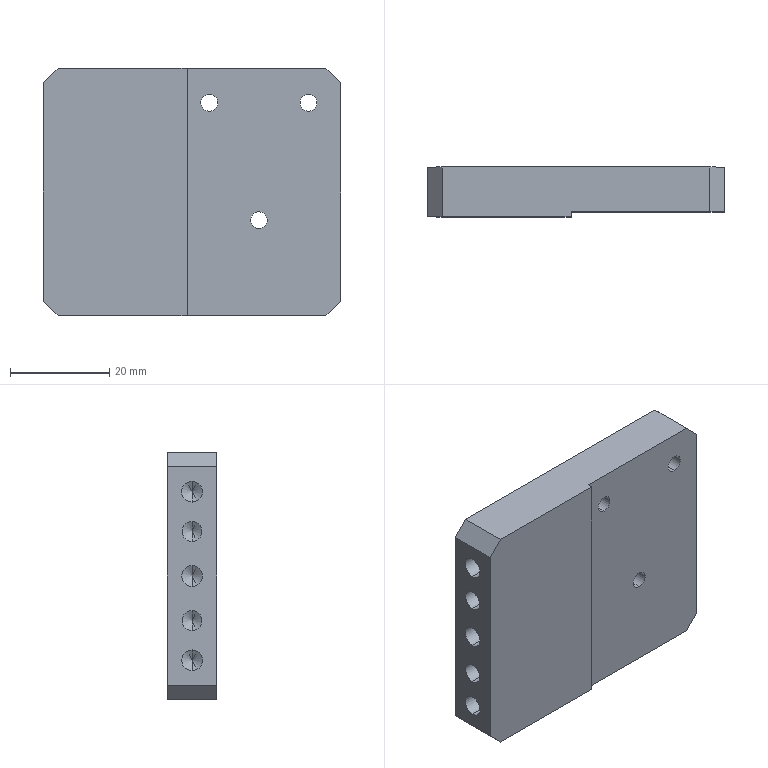Part | SolidWorks | features HoleWzd 3, Chamfer 1, Extrusion 1, ICE 1 | 1 solid | 47 faces | box 60 x 10 x 50 mm | volume 26983 mm3 | cylinder 22 | plane 15 | cone 10 | commonest cylinder face diameters 3.4 x6 4.2 x6 6 x6 4 x4
STEP:
#1=CARTESIAN_POINT('',(-17.6,5.,7.));
#2=VERTEX_POINT('',#1);
#3=CARTESIAN_POINT('',(-17.6,5.,11.));
#4=VERTEX_POINT('',#3);
#5=CARTESIAN_POINT('',(-17.6,5.,9.));
#6=DIRECTION('',(-1.,0.,0.));
#7=DIRECTION('',(0.,0.,1.));
#8=AXIS2_PLACEMENT_3D('',#5,#6,#7);
#9=CIRCLE('',#8,2.);
#10=EDGE_CURVE('',#2,#4,#9,.T.);
#11=ORIENTED_EDGE('',*,*,#10,.F.);
#12=CARTESIAN_POINT('',(-30.,5.,7.));
#13=VERTEX_POINT('',#12);
#14=CARTESIAN_POINT('',(-30.,5.,7.));
#15=DIRECTION('',(-1.,0.,0.));
#16=VECTOR('',#15,1000.);
#17=LINE('',#14,#16);
#18=EDGE_CURVE('',#2,#13,#17,.T.);
#19=ORIENTED_EDGE('',*,*,#18,.T.);
#20=CARTESIAN_POINT('',(-30.,5.,11.));
#21=VERTEX_POINT('',#20);
#22=CARTESIAN_POINT('',(-30.,5.,9.));
#23=DIRECTION('',(-1.,0.,0.));
#24=DIRECTION('',(0.,0.,1.));
#25=AXIS2_PLACEMENT_3D('',#22,#23,#24);
#26=CIRCLE('',#25,2.);
#27=EDGE_CURVE('',#13,#21,#26,.T.);
#28=ORIENTED_EDGE('',*,*,#27,.T.);
#29=CARTESIAN_POINT('',(-30.,5.,11.));
#30=DIRECTION('',(-1.,0.,0.));
#31=VECTOR('',#30,1000.);
#32=LINE('',#29,#31);
#33=EDGE_CURVE('',#4,#21,#32,.T.);
#34=ORIENTED_EDGE('',*,*,#33,.F.);
#35=EDGE_LOOP('',(#11,#19,#28,#34));
#36=FACE_OUTER_BOUND('',#35,.T.);
#37=CARTESIAN_POINT('',(-30.,5.,9.));
#38=DIRECTION('',(-1.,0.,0.));
#39=DIRECTION('',(0.,0.,1.));
#40=AXIS2_PLACEMENT_3D('',#37,#38,#39);
#41=CYLINDRICAL_SURFACE('',#40,2.);
#42=ADVANCED_FACE('',(#36),#41,.F.);
#43=CARTESIAN_POINT('',(-16.398,5.,9.));
#44=VERTEX_POINT('',#43);
#45=CARTESIAN_POINT('',(-17.6,5.,11.));
#46=DIRECTION('',(-0.515,0.,0.8572));
#47=VECTOR('',#46,1000.);
#48=LINE('',#45,#47);
#49=EDGE_CURVE('',#44,#4,#48,.T.);
#50=ORIENTED_EDGE('',*,*,#49,.F.);
#51=CARTESIAN_POINT('',(-17.6,5.,7.));
#52=DIRECTION('',(-0.515,0.,-0.8572));
#53=VECTOR('',#52,1000.);
#54=LINE('',#51,#53);
#55=EDGE_CURVE('',#44,#2,#54,.T.);
#56=ORIENTED_EDGE('',*,*,#55,.T.);
#57=ORIENTED_EDGE('',*,*,#10,.T.);
#58=EDGE_LOOP('',(#50,#56,#57));
#59=FACE_OUTER_BOUND('',#58,.T.);
#60=CARTESIAN_POINT('',(-17.6,5.,9.));
#61=DIRECTION('',(-1.,0.,0.));
#62=DIRECTION('',(0.,0.,1.));
#63=AXIS2_PLACEMENT_3D('',#60,#61,#62);
#64=CONICAL_SURFACE('',#63,2.,1.03);
#65=ADVANCED_FACE('',(#59),#64,.F.);
#66=CARTESIAN_POINT('',(-17.6,5.,-11.));
#67=VERTEX_POINT('',#66);
#68=CARTESIAN_POINT('',(-17.6,5.,-7.));
#69=VERTEX_POINT('',#68);
#70=CARTESIAN_POINT('',(-17.6,5.,-9.));
#71=DIRECTION('',(-1.,0.,0.));
#72=DIRECTION('',(0.,0.,1.));
#73=AXIS2_PLACEMENT_3D('',#70,#71,#72);
#74=CIRCLE('',#73,2.);
#75=EDGE_CURVE('',#67,#69,#74,.T.);
#76=ORIENTED_EDGE('',*,*,#75,.F.);
#77=CARTESIAN_POINT('',(-30.,5.,-11.));
#78=VERTEX_POINT('',#77);
#79=CARTESIAN_POINT('',(-30.,5.,-11.));
#80=DIRECTION('',(-1.,0.,0.));
#81=VECTOR('',#80,1000.);
#82=LINE('',#79,#81);
#83=EDGE_CURVE('',#67,#78,#82,.T.);
#84=ORIENTED_EDGE('',*,*,#83,.T.);
#85=CARTESIAN_POINT('',(-30.,5.,-7.));
#86=VERTEX_POINT('',#85);
#87=CARTESIAN_POINT('',(-30.,5.,-9.));
#88=DIRECTION('',(-1.,0.,0.));
#89=DIRECTION('',(0.,0.,1.));
#90=AXIS2_PLACEMENT_3D('',#87,#88,#89);
#91=CIRCLE('',#90,2.);
#92=EDGE_CURVE('',#78,#86,#91,.T.);
#93=ORIENTED_EDGE('',*,*,#92,.T.);
#94=CARTESIAN_POINT('',(-30.,5.,-7.));
#95=DIRECTION('',(-1.,0.,0.));
#96=VECTOR('',#95,1000.);
#97=LINE('',#94,#96);
#98=EDGE_CURVE('',#69,#86,#97,.T.);
#99=ORIENTED_EDGE('',*,*,#98,.F.);
#100=EDGE_LOOP('',(#76,#84,#93,#99));
#101=FACE_OUTER_BOUND('',#100,.T.);
#102=CARTESIAN_POINT('',(-30.,5.,-9.));
#103=DIRECTION('',(-1.,0.,0.));
#104=DIRECTION('',(0.,0.,1.));
#105=AXIS2_PLACEMENT_3D('',#102,#103,#104);
#106=CYLINDRICAL_SURFACE('',#105,2.);
#107=ADVANCED_FACE('',(#101),#106,.F.);
#108=CARTESIAN_POINT('',(-16.398,5.,-9.));
#109=VERTEX_POINT('',#108);
#110=CARTESIAN_POINT('',(-17.6,5.,-7.));
#111=DIRECTION('',(-0.515,0.,0.8572));
#112=VECTOR('',#111,1000.);
#113=LINE('',#110,#112);
#114=EDGE_CURVE('',#109,#69,#113,.T.);
#115=ORIENTED_EDGE('',*,*,#114,.F.);
#116=CARTESIAN_POINT('',(-17.6,5.,-11.));
#117=DIRECTION('',(-0.515,0.,-0.8572));
#118=VECTOR('',#117,1000.);
#119=LINE('',#116,#118);
#120=EDGE_CURVE('',#109,#67,#119,.T.);
#121=ORIENTED_EDGE('',*,*,#120,.T.);
#122=ORIENTED_EDGE('',*,*,#75,.T.);
#123=EDGE_LOOP('',(#115,#121,#122));
#124=FACE_OUTER_BOUND('',#123,.T.);
#125=CARTESIAN_POINT('',(-17.6,5.,-9.));
#126=DIRECTION('',(-1.,0.,0.));
#127=DIRECTION('',(0.,0.,1.));
#128=AXIS2_PLACEMENT_3D('',#125,#126,#127);
#129=CONICAL_SURFACE('',#128,2.,1.03);
#130=ADVANCED_FACE('',(#124),#129,.F.);
#131=CARTESIAN_POINT('',(23.5,6.6,15.));
#132=VERTEX_POINT('',#131);
#133=CARTESIAN_POINT('',(23.5,6.6,21.));
#134=VERTEX_POINT('',#133);
#135=CARTESIAN_POINT('',(23.5,6.6,18.));
#136=DIRECTION('',(0.,1.,0.));
#137=DIRECTION('',(0.,0.,1.));
#138=AXIS2_PLACEMENT_3D('',#135,#136,#137);
#139=CIRCLE('',#138,3.);
#140=EDGE_CURVE('',#132,#134,#139,.T.);
#141=ORIENTED_EDGE('',*,*,#140,.F.);
#142=CARTESIAN_POINT('',(23.5,10.,15.));
#143=VERTEX_POINT('',#142);
#144=CARTESIAN_POINT('',(23.5,10.,15.));
#145=DIRECTION('',(0.,1.,0.));
#146=VECTOR('',#145,1000.);
#147=LINE('',#144,#146);
#148=EDGE_CURVE('',#132,#143,#147,.T.);
#149=ORIENTED_EDGE('',*,*,#148,.T.);
#150=CARTESIAN_POINT('',(23.5,10.,21.));
#151=VERTEX_POINT('',#150);
#152=CARTESIAN_POINT('',(23.5,10.,18.));
#153=DIRECTION('',(0.,1.,0.));
#154=DIRECTION('',(0.,0.,1.));
#155=AXIS2_PLACEMENT_3D('',#152,#153,#154);
#156=CIRCLE('',#155,3.);
#157=EDGE_CURVE('',#143,#151,#156,.T.);
#158=ORIENTED_EDGE('',*,*,#157,.T.);
#159=CARTESIAN_POINT('',(23.5,10.,21.));
#160=DIRECTION('',(0.,1.,0.));
#161=VECTOR('',#160,1000.);
#162=LINE('',#159,#161);
#163=EDGE_CURVE('',#134,#151,#162,.T.);
#164=ORIENTED_EDGE('',*,*,#163,.F.);
#165=EDGE_LOOP('',(#141,#149,#158,#164));
#166=FACE_OUTER_BOUND('',#165,.T.);
#167=CARTESIAN_POINT('',(23.5,10.,18.));
#168=DIRECTION('',(0.,1.,0.));
#169=DIRECTION('',(0.,0.,1.));
#170=AXIS2_PLACEMENT_3D('',#167,#168,#169);
#171=CYLINDRICAL_SURFACE('',#170,3.);
#172=ADVANCED_FACE('',(#166),#171,.F.);
#173=CARTESIAN_POINT('',(23.5,1.,19.7));
#174=VERTEX_POINT('',#173);
#175=CARTESIAN_POINT('',(23.5,1.,16.3));
#176=VERTEX_POINT('',#175);
#177=CARTESIAN_POINT('',(23.5,1.,18.));
#178=DIRECTION('',(0.,-1.,0.));
#179=DIRECTION('',(0.,0.,-1.));
#180=AXIS2_PLACEMENT_3D('',#177,#178,#179);
#181=CIRCLE('',#180,1.7);
#182=EDGE_CURVE('',#174,#176,#181,.T.);
#183=ORIENTED_EDGE('',*,*,#182,.T.);
#184=CARTESIAN_POINT('',(23.5,6.6,16.3));
#185=VERTEX_POINT('',#184);
#186=CARTESIAN_POINT('',(23.5,10.,16.3));
#187=DIRECTION('',(0.,1.,0.));
#188=VECTOR('',#187,1000.);
#189=LINE('',#186,#188);
#190=EDGE_CURVE('',#176,#185,#189,.T.);
#191=ORIENTED_EDGE('',*,*,#190,.T.);
#192=CARTESIAN_POINT('',(23.5,6.6,19.7));
#193=VERTEX_POINT('',#192);
#194=CARTESIAN_POINT('',(23.5,6.6,18.));
#195=DIRECTION('',(0.,1.,0.));
#196=DIRECTION('',(0.,0.,1.));
#197=AXIS2_PLACEMENT_3D('',#194,#195,#196);
#198=CIRCLE('',#197,1.7);
#199=EDGE_CURVE('',#185,#193,#198,.T.);
#200=ORIENTED_EDGE('',*,*,#199,.T.);
#201=CARTESIAN_POINT('',(23.5,10.,19.7));
#202=DIRECTION('',(0.,1.,0.));
#203=VECTOR('',#202,1000.);
#204=LINE('',#201,#203);
#205=EDGE_CURVE('',#174,#193,#204,.T.);
#206=ORIENTED_EDGE('',*,*,#205,.F.);
#207=EDGE_LOOP('',(#183,#191,#200,#206));
#208=FACE_OUTER_BOUND('',#207,.T.);
#209=CARTESIAN_POINT('',(23.5,10.,18.));
#210=DIRECTION('',(0.,1.,0.));
#211=DIRECTION('',(0.,0.,1.));
#212=AXIS2_PLACEMENT_3D('',#209,#210,#211);
#213=CYLINDRICAL_SURFACE('',#212,1.7);
#214=ADVANCED_FACE('',(#208),#213,.F.);
#215=CARTESIAN_POINT('',(3.5,6.6,15.));
#216=VERTEX_POINT('',#215);
#217=CARTESIAN_POINT('',(3.5,6.6,21.));
#218=VERTEX_POINT('',#217);
#219=CARTESIAN_POINT('',(3.5,6.6,18.));
#220=DIRECTION('',(0.,1.,0.));
#221=DIRECTION('',(0.,0.,1.));
#222=AXIS2_PLACEMENT_3D('',#219,#220,#221);
#223=CIRCLE('',#222,3.);
#224=EDGE_CURVE('',#216,#218,#223,.T.);
#225=ORIENTED_EDGE('',*,*,#224,.F.);
#226=CARTESIAN_POINT('',(3.5,10.,15.));
#227=VERTEX_POINT('',#226);
#228=CARTESIAN_POINT('',(3.5,10.,15.));
#229=DIRECTION('',(0.,1.,0.));
#230=VECTOR('',#229,1000.);
#231=LINE('',#228,#230);
#232=EDGE_CURVE('',#216,#227,#231,.T.);
#233=ORIENTED_EDGE('',*,*,#232,.T.);
#234=CARTESIAN_POINT('',(3.5,10.,21.));
#235=VERTEX_POINT('',#234);
#236=CARTESIAN_POINT('',(3.5,10.,18.));
#237=DIRECTION('',(0.,1.,0.));
#238=DIRECTION('',(0.,0.,1.));
#239=AXIS2_PLACEMENT_3D('',#236,#237,#238);
#240=CIRCLE('',#239,3.);
#241=EDGE_CURVE('',#227,#235,#240,.T.);
#242=ORIENTED_EDGE('',*,*,#241,.T.);
#243=CARTESIAN_POINT('',(3.5,10.,21.));
#244=DIRECTION('',(0.,1.,0.));
#245=VECTOR('',#244,1000.);
#246=LINE('',#243,#245);
#247=EDGE_CURVE('',#218,#235,#246,.T.);
#248=ORIENTED_EDGE('',*,*,#247,.F.);
#249=EDGE_LOOP('',(#225,#233,#242,#248));
#250=FACE_OUTER_BOUND('',#249,.T.);
#251=CARTESIAN_POINT('',(3.5,10.,18.));
#252=DIRECTION('',(0.,1.,0.));
#253=DIRECTION('',(0.,0.,1.));
#254=AXIS2_PLACEMENT_3D('',#251,#252,#253);
#255=CYLINDRICAL_SURFACE('',#254,3.);
#256=ADVANCED_FACE('',(#250),#255,.F.);
#257=CARTESIAN_POINT('',(3.5,1.,19.7));
#258=VERTEX_POINT('',#257);
#259=CARTESIAN_POINT('',(3.5,1.,16.3));
#260=VERTEX_POINT('',#259);
#261=CARTESIAN_POINT('',(3.5,1.,18.));
#262=DIRECTION('',(0.,-1.,0.));
#263=DIRECTION('',(0.,0.,-1.));
#264=AXIS2_PLACEMENT_3D('',#261,#262,#263);
#265=CIRCLE('',#264,1.7);
#266=EDGE_CURVE('',#258,#260,#265,.T.);
#267=ORIENTED_EDGE('',*,*,#266,.T.);
#268=CARTESIAN_POINT('',(3.5,6.6,16.3));
#269=VERTEX_POINT('',#268);
#270=CARTESIAN_POINT('',(3.5,10.,16.3));
#271=DIRECTION('',(0.,1.,0.));
#272=VECTOR('',#271,1000.);
#273=LINE('',#270,#272);
#274=EDGE_CURVE('',#260,#269,#273,.T.);
#275=ORIENTED_EDGE('',*,*,#274,.T.);
#276=CARTESIAN_POINT('',(3.5,6.6,19.7));
#277=VERTEX_POINT('',#276);
#278=CARTESIAN_POINT('',(3.5,6.6,18.));
#279=DIRECTION('',(0.,1.,0.));
#280=DIRECTION('',(0.,0.,1.));
#281=AXIS2_PLACEMENT_3D('',#278,#279,#280);
#282=CIRCLE('',#281,1.7);
#283=EDGE_CURVE('',#269,#277,#282,.T.);
#284=ORIENTED_EDGE('',*,*,#283,.T.);
#285=CARTESIAN_POINT('',(3.5,10.,19.7));
#286=DIRECTION('',(0.,1.,0.));
#287=VECTOR('',#286,1000.);
#288=LINE('',#285,#287);
#289=EDGE_CURVE('',#258,#277,#288,.T.);
#290=ORIENTED_EDGE('',*,*,#289,.F.);
#291=EDGE_LOOP('',(#267,#275,#284,#290));
#292=FACE_OUTER_BOUND('',#291,.T.);
#293=CARTESIAN_POINT('',(3.5,10.,18.));
#294=DIRECTION('',(0.,1.,0.));
#295=DIRECTION('',(0.,0.,1.));
#296=AXIS2_PLACEMENT_3D('',#293,#294,#295);
#297=CYLINDRICAL_SURFACE('',#296,1.7);
#298=ADVANCED_FACE('',(#292),#297,.F.);
#299=CARTESIAN_POINT('',(13.5,6.6,-8.7));
#300=VERTEX_POINT('',#299);
#301=CARTESIAN_POINT('',(13.5,6.6,-2.7));
#302=VERTEX_POINT('',#301);
#303=CARTESIAN_POINT('',(13.5,6.6,-5.7));
#304=DIRECTION('',(0.,1.,0.));
#305=DIRECTION('',(0.,0.,1.));
#306=AXIS2_PLACEMENT_3D('',#303,#304,#305);
#307=CIRCLE('',#306,3.);
#308=EDGE_CURVE('',#300,#302,#307,.T.);
#309=ORIENTED_EDGE('',*,*,#308,.F.);
#310=CARTESIAN_POINT('',(13.5,10.,-8.7));
#311=VERTEX_POINT('',#310);
#312=CARTESIAN_POINT('',(13.5,10.,-8.7));
#313=DIRECTION('',(0.,1.,0.));
#314=VECTOR('',#313,1000.);
#315=LINE('',#312,#314);
#316=EDGE_CURVE('',#300,#311,#315,.T.);
#317=ORIENTED_EDGE('',*,*,#316,.T.);
#318=CARTESIAN_POINT('',(13.5,10.,-2.7));
#319=VERTEX_POINT('',#318);
#320=CARTESIAN_POINT('',(13.5,10.,-5.7));
#321=DIRECTION('',(0.,1.,0.));
#322=DIRECTION('',(0.,0.,1.));
#323=AXIS2_PLACEMENT_3D('',#320,#321,#322);
#324=CIRCLE('',#323,3.);
#325=EDGE_CURVE('',#311,#319,#324,.T.);
#326=ORIENTED_EDGE('',*,*,#325,.T.);
#327=CARTESIAN_POINT('',(13.5,10.,-2.7));
#328=DIRECTION('',(0.,1.,0.));
#329=VECTOR('',#328,1000.);
#330=LINE('',#327,#329);
#331=EDGE_CURVE('',#302,#319,#330,.T.);
#332=ORIENTED_EDGE('',*,*,#331,.F.);
#333=EDGE_LOOP('',(#309,#317,#326,#332));
#334=FACE_OUTER_BOUND('',#333,.T.);
#335=CARTESIAN_POINT('',(13.5,10.,-5.7));
#336=DIRECTION('',(0.,1.,0.));
#337=DIRECTION('',(0.,0.,1.));
#338=AXIS2_PLACEMENT_3D('',#335,#336,#337);
#339=CYLINDRICAL_SURFACE('',#338,3.);
#340=ADVANCED_FACE('',(#334),#339,.F.);
#341=CARTESIAN_POINT('',(13.5,1.,-4.));
#342=VERTEX_POINT('',#341);
#343=CARTESIAN_POINT('',(13.5,1.,-7.4));
#344=VERTEX_POINT('',#343);
#345=CARTESIAN_POINT('',(13.5,1.,-5.7));
#346=DIRECTION('',(0.,-1.,0.));
#347=DIRECTION('',(0.,0.,-1.));
#348=AXIS2_PLACEMENT_3D('',#345,#346,#347);
#349=CIRCLE('',#348,1.7);
#350=EDGE_CURVE('',#342,#344,#349,.T.);
#351=ORIENTED_EDGE('',*,*,#350,.T.);
#352=CARTESIAN_POINT('',(13.5,6.6,-7.4));
#353=VERTEX_POINT('',#352);
#354=CARTESIAN_POINT('',(13.5,10.,-7.4));
#355=DIRECTION('',(0.,1.,0.));
#356=VECTOR('',#355,1000.);
#357=LINE('',#354,#356);
#358=EDGE_CURVE('',#344,#353,#357,.T.);
#359=ORIENTED_EDGE('',*,*,#358,.T.);
#360=CARTESIAN_POINT('',(13.5,6.6,-4.));
#361=VERTEX_POINT('',#360);
#362=CARTESIAN_POINT('',(13.5,6.6,-5.7));
#363=DIRECTION('',(0.,1.,0.));
#364=DIRECTION('',(0.,0.,1.));
#365=AXIS2_PLACEMENT_3D('',#362,#363,#364);
#366=CIRCLE('',#365,1.7);
#367=EDGE_CURVE('',#353,#361,#366,.T.);
#368=ORIENTED_EDGE('',*,*,#367,.T.);
#369=CARTESIAN_POINT('',(13.5,10.,-4.));
#370=DIRECTION('',(0.,1.,0.));
#371=VECTOR('',#370,1000.);
#372=LINE('',#369,#371);
#373=EDGE_CURVE('',#342,#361,#372,.T.);
#374=ORIENTED_EDGE('',*,*,#373,.F.);
#375=EDGE_LOOP('',(#351,#359,#368,#374));
#376=FACE_OUTER_BOUND('',#375,.T.);
#377=CARTESIAN_POINT('',(13.5,10.,-5.7));
#378=DIRECTION('',(0.,1.,0.));
#379=DIRECTION('',(0.,0.,1.));
#380=AXIS2_PLACEMENT_3D('',#377,#378,#379);
#381=CYLINDRICAL_SURFACE('',#380,1.7);
#382=ADVANCED_FACE('',(#376),#381,.F.);
#383=CARTESIAN_POINT('',(-17.6,5.,14.9));
#384=VERTEX_POINT('',#383);
#385=CARTESIAN_POINT('',(-17.6,5.,19.1));
#386=VERTEX_POINT('',#385);
#387=CARTESIAN_POINT('',(-17.6,5.,17.));
#388=DIRECTION('',(-1.,0.,0.));
#389=DIRECTION('',(0.,0.,1.));
#390=AXIS2_PLACEMENT_3D('',#387,#388,#389);
#391=CIRCLE('',#390,2.1);
#392=EDGE_CURVE('',#384,#386,#391,.T.);
#393=ORIENTED_EDGE('',*,*,#392,.F.);
#394=CARTESIAN_POINT('',(-30.,5.,14.9));
#395=VERTEX_POINT('',#394);
#396=CARTESIAN_POINT('',(-30.,5.,14.9));
#397=DIRECTION('',(-1.,0.,0.));
#398=VECTOR('',#397,1000.);
#399=LINE('',#396,#398);
#400=EDGE_CURVE('',#384,#395,#399,.T.);
#401=ORIENTED_EDGE('',*,*,#400,.T.);
#402=CARTESIAN_POINT('',(-30.,5.,19.1));
#403=VERTEX_POINT('',#402);
#404=CARTESIAN_POINT('',(-30.,5.,17.));
#405=DIRECTION('',(-1.,0.,0.));
#406=DIRECTION('',(0.,0.,1.));
#407=AXIS2_PLACEMENT_3D('',#404,#405,#406);
#408=CIRCLE('',#407,2.1);
#409=EDGE_CURVE('',#395,#403,#408,.T.);
#410=ORIENTED_EDGE('',*,*,#409,.T.);
#411=CARTESIAN_POINT('',(-30.,5.,19.1));
#412=DIRECTION('',(-1.,0.,0.));
#413=VECTOR('',#412,1000.);
#414=LINE('',#411,#413);
#415=EDGE_CURVE('',#386,#403,#414,.T.);
#416=ORIENTED_EDGE('',*,*,#415,.F.);
#417=EDGE_LOOP('',(#393,#401,#410,#416));
#418=FACE_OUTER_BOUND('',#417,.T.);
#419=CARTESIAN_POINT('',(-30.,5.,17.));
#420=DIRECTION('',(-1.,0.,0.));
#421=DIRECTION('',(0.,0.,1.));
#422=AXIS2_PLACEMENT_3D('',#419,#420,#421);
#423=CYLINDRICAL_SURFACE('',#422,2.1);
#424=ADVANCED_FACE('',(#418),#423,.F.);
#425=CARTESIAN_POINT('',(-16.338,5.,17.));
#426=VERTEX_POINT('',#425);
#427=CARTESIAN_POINT('',(-17.6,5.,19.1));
#428=DIRECTION('',(-0.515,0.,0.8572));
#429=VECTOR('',#428,1000.);
#430=LINE('',#427,#429);
#431=EDGE_CURVE('',#426,#386,#430,.T.);
#432=ORIENTED_EDGE('',*,*,#431,.F.);
#433=CARTESIAN_POINT('',(-17.6,5.,14.9));
#434=DIRECTION('',(-0.515,0.,-0.8572));
#435=VECTOR('',#434,1000.);
#436=LINE('',#433,#435);
#437=EDGE_CURVE('',#426,#384,#436,.T.);
#438=ORIENTED_EDGE('',*,*,#437,.T.);
#439=ORIENTED_EDGE('',*,*,#392,.T.);
#440=EDGE_LOOP('',(#432,#438,#439));
#441=FACE_OUTER_BOUND('',#440,.T.);
#442=CARTESIAN_POINT('',(-17.6,5.,17.));
#443=DIRECTION('',(-1.,0.,0.));
#444=DIRECTION('',(0.,0.,1.));
#445=AXIS2_PLACEMENT_3D('',#442,#443,#444);
#446=CONICAL_SURFACE('',#445,2.1,1.03);
#447=ADVANCED_FACE('',(#441),#446,.F.);
#448=CARTESIAN_POINT('',(-17.6,4.974,-19.1));
#449=VERTEX_POINT('',#448);
#450=CARTESIAN_POINT('',(-17.6,4.974,-14.9));
#451=VERTEX_POINT('',#450);
#452=CARTESIAN_POINT('',(-17.6,4.974,-17.));
#453=DIRECTION('',(-1.,0.,0.));
#454=DIRECTION('',(0.,0.,1.));
#455=AXIS2_PLACEMENT_3D('',#452,#453,#454);
#456=CIRCLE('',#455,2.1);
#457=EDGE_CURVE('',#449,#451,#456,.T.);
#458=ORIENTED_EDGE('',*,*,#457,.F.);
#459=CARTESIAN_POINT('',(-30.,4.974,-19.1));
#460=VERTEX_POINT('',#459);
#461=CARTESIAN_POINT('',(-30.,4.974,-19.1));
#462=DIRECTION('',(-1.,0.,0.));
#463=VECTOR('',#462,1000.);
#464=LINE('',#461,#463);
#465=EDGE_CURVE('',#449,#460,#464,.T.);
#466=ORIENTED_EDGE('',*,*,#465,.T.);
#467=CARTESIAN_POINT('',(-30.,4.974,-14.9));
#468=VERTEX_POINT('',#467);
#469=CARTESIAN_POINT('',(-30.,4.974,-17.));
#470=DIRECTION('',(-1.,0.,0.));
#471=DIRECTION('',(0.,0.,1.));
#472=AXIS2_PLACEMENT_3D('',#469,#470,#471);
#473=CIRCLE('',#472,2.1);
#474=EDGE_CURVE('',#460,#468,#473,.T.);
#475=ORIENTED_EDGE('',*,*,#474,.T.);
#476=CARTESIAN_POINT('',(-30.,4.974,-14.9));
#477=DIRECTION('',(-1.,0.,0.));
#478=VECTOR('',#477,1000.);
#479=LINE('',#476,#478);
#480=EDGE_CURVE('',#451,#468,#479,.T.);
#481=ORIENTED_EDGE('',*,*,#480,.F.);
#482=EDGE_LOOP('',(#458,#466,#475,#481));
#483=FACE_OUTER_BOUND('',#482,.T.);
#484=CARTESIAN_POINT('',(-30.,4.974,-17.));
#485=DIRECTION('',(-1.,0.,0.));
#486=DIRECTION('',(0.,0.,1.));
#487=AXIS2_PLACEMENT_3D('',#484,#485,#486);
#488=CYLINDRICAL_SURFACE('',#487,2.1);
#489=ADVANCED_FACE('',(#483),#488,.F.);
#490=CARTESIAN_POINT('',(-16.338,4.974,-17.));
#491=VERTEX_POINT('',#490);
#492=CARTESIAN_POINT('',(-17.6,4.974,-14.9));
#493=DIRECTION('',(-0.515,0.,0.8572));
#494=VECTOR('',#493,1000.);
#495=LINE('',#492,#494);
#496=EDGE_CURVE('',#491,#451,#495,.T.);
#497=ORIENTED_EDGE('',*,*,#496,.F.);
#498=CARTESIAN_POINT('',(-17.6,4.974,-19.1));
#499=DIRECTION('',(-0.515,0.,-0.8572));
#500=VECTOR('',#499,1000.);
#501=LINE('',#498,#500);
#502=EDGE_CURVE('',#491,#449,#501,.T.);
#503=ORIENTED_EDGE('',*,*,#502,.T.);
#504=ORIENTED_EDGE('',*,*,#457,.T.);
#505=EDGE_LOOP('',(#497,#503,#504));
#506=FACE_OUTER_BOUND('',#505,.T.);
#507=CARTESIAN_POINT('',(-17.6,4.974,-17.));
#508=DIRECTION('',(-1.,0.,0.));
#509=DIRECTION('',(0.,0.,1.));
#510=AXIS2_PLACEMENT_3D('',#507,#508,#509);
#511=CONICAL_SURFACE('',#510,2.1,1.03);
#512=ADVANCED_FACE('',(#506),#511,.F.);
#513=CARTESIAN_POINT('',(-17.6,4.974,-2.1));
#514=VERTEX_POINT('',#513);
#515=CARTESIAN_POINT('',(-17.6,4.974,2.1));
#516=VERTEX_POINT('',#515);
#517=CARTESIAN_POINT('',(-17.6,4.974,0.));
#518=DIRECTION('',(-1.,0.,0.));
#519=DIRECTION('',(0.,0.,1.));
#520=AXIS2_PLACEMENT_3D('',#517,#518,#519);
#521=CIRCLE('',#520,2.1);
#522=EDGE_CURVE('',#514,#516,#521,.T.);
#523=ORIENTED_EDGE('',*,*,#522,.F.);
#524=CARTESIAN_POINT('',(-30.,4.974,-2.1));
#525=VERTEX_POINT('',#524);
#526=CARTESIAN_POINT('',(-30.,4.974,-2.1));
#527=DIRECTION('',(-1.,0.,0.));
#528=VECTOR('',#527,1000.);
#529=LINE('',#526,#528);
#530=EDGE_CURVE('',#514,#525,#529,.T.);
#531=ORIENTED_EDGE('',*,*,#530,.T.);
#532=CARTESIAN_POINT('',(-30.,4.974,2.1));
#533=VERTEX_POINT('',#532);
#534=CARTESIAN_POINT('',(-30.,4.974,0.));
#535=DIRECTION('',(-1.,0.,0.));
#536=DIRECTION('',(0.,0.,1.));
#537=AXIS2_PLACEMENT_3D('',#534,#535,#536);
#538=CIRCLE('',#537,2.1);
#539=EDGE_CURVE('',#525,#533,#538,.T.);
#540=ORIENTED_EDGE('',*,*,#539,.T.);
#541=CARTESIAN_POINT('',(-30.,4.974,2.1));
#542=DIRECTION('',(-1.,0.,0.));
#543=VECTOR('',#542,1000.);
#544=LINE('',#541,#543);
#545=EDGE_CURVE('',#516,#533,#544,.T.);
#546=ORIENTED_EDGE('',*,*,#545,.F.);
#547=EDGE_LOOP('',(#523,#531,#540,#546));
#548=FACE_OUTER_BOUND('',#547,.T.);
#549=CARTESIAN_POINT('',(-30.,4.974,0.));
#550=DIRECTION('',(-1.,0.,0.));
#551=DIRECTION('',(0.,0.,1.));
#552=AXIS2_PLACEMENT_3D('',#549,#550,#551);
#553=CYLINDRICAL_SURFACE('',#552,2.1);
#554=ADVANCED_FACE('',(#548),#553,.F.);
#555=CARTESIAN_POINT('',(-16.338,4.974,0.));
#556=VERTEX_POINT('',#555);
#557=CARTESIAN_POINT('',(-17.6,4.974,2.1));
#558=DIRECTION('',(-0.515,0.,0.8572));
#559=VECTOR('',#558,1000.);
#560=LINE('',#557,#559);
#561=EDGE_CURVE('',#556,#516,#560,.T.);
#562=ORIENTED_EDGE('',*,*,#561,.F.);
#563=CARTESIAN_POINT('',(-17.6,4.974,-2.1));
#564=DIRECTION('',(-0.515,0.,-0.8572));
#565=VECTOR('',#564,1000.);
#566=LINE('',#563,#565);
#567=EDGE_CURVE('',#556,#514,#566,.T.);
#568=ORIENTED_EDGE('',*,*,#567,.T.);
#569=ORIENTED_EDGE('',*,*,#522,.T.);
#570=EDGE_LOOP('',(#562,#568,#569));
#571=FACE_OUTER_BOUND('',#570,.T.);
#572=CARTESIAN_POINT('',(-17.6,4.974,0.));
#573=DIRECTION('',(-1.,0.,0.));
#574=DIRECTION('',(0.,0.,1.));
#575=AXIS2_PLACEMENT_3D('',#572,#573,#574);
#576=CONICAL_SURFACE('',#575,2.1,1.03);
#577=ADVANCED_FACE('',(#571),#576,.F.);
#578=CARTESIAN_POINT('',(30.,1.,-22.));
#579=VERTEX_POINT('',#578);
#580=CARTESIAN_POINT('',(30.,1.,22.));
#581=VERTEX_POINT('',#580);
#582=CARTESIAN_POINT('',(30.,1.,25.));
#583=DIRECTION('',(0.,0.,1.));
#584=VECTOR('',#583,1000.);
#585=LINE('',#582,#584);
#586=EDGE_CURVE('',#579,#581,#585,.T.);
#587=ORIENTED_EDGE('',*,*,#586,.F.);
#588=CARTESIAN_POINT('',(30.,10.,-22.));
#589=VERTEX_POINT('',#588);
#590=CARTESIAN_POINT('',(30.,10.,-22.));
#591=DIRECTION('',(0.,1.,0.));
#592=VECTOR('',#591,1000.);
#593=LINE('',#590,#592);
#594=EDGE_CURVE('',#579,#589,#593,.T.);
#595=ORIENTED_EDGE('',*,*,#594,.T.);
#596=CARTESIAN_POINT('',(30.,10.,22.));
#597=VERTEX_POINT('',#596);
#598=CARTESIAN_POINT('',(30.,10.,-25.));
#599=DIRECTION('',(0.,0.,-1.));
#600=VECTOR('',#599,1000.);
#601=LINE('',#598,#600);
#602=EDGE_CURVE('',#597,#589,#601,.T.);
#603=ORIENTED_EDGE('',*,*,#602,.F.);
#604=CARTESIAN_POINT('',(30.,10.,22.));
#605=DIRECTION('',(0.,-1.,0.));
#606=VECTOR('',#605,1000.);
#607=LINE('',#604,#606);
#608=EDGE_CURVE('',#597,#581,#607,.T.);
#609=ORIENTED_EDGE('',*,*,#608,.T.);
#610=EDGE_LOOP('',(#587,#595,#603,#609));
#611=FACE_OUTER_BOUND('',#610,.T.);
#612=CARTESIAN_POINT('',(30.,10.,-25.));
#613=DIRECTION('',(-1.,0.,0.));
#614=DIRECTION('',(0.,0.,1.));
#615=AXIS2_PLACEMENT_3D('',#612,#613,#614);
#616=PLANE('',#615);
#617=ADVANCED_FACE('',(#611),#616,.F.);
#618=CARTESIAN_POINT('',(-1.,0.,-25.));
#619=VERTEX_POINT('',#618);
#620=CARTESIAN_POINT('',(-27.,0.,-25.));
#621=VERTEX_POINT('',#620);
#622=CARTESIAN_POINT('',(-30.,0.,-25.));
#623=DIRECTION('',(-1.,0.,0.));
#624=VECTOR('',#623,1000.);
#625=LINE('',#622,#624);
#626=EDGE_CURVE('',#619,#621,#625,.T.);
#627=ORIENTED_EDGE('',*,*,#626,.T.);
#628=CARTESIAN_POINT('',(-27.,10.,-25.));
#629=VERTEX_POINT('',#628);
#630=CARTESIAN_POINT('',(-27.,10.,-25.));
#631=DIRECTION('',(0.,1.,0.));
#632=VECTOR('',#631,1000.);
#633=LINE('',#630,#632);
#634=EDGE_CURVE('',#621,#629,#633,.T.);
#635=ORIENTED_EDGE('',*,*,#634,.T.);
#636=CARTESIAN_POINT('',(27.,10.,-25.));
#637=VERTEX_POINT('',#636);
#638=CARTESIAN_POINT('',(-30.,10.,-25.));
#639=DIRECTION('',(-1.,0.,0.));
#640=VECTOR('',#639,1000.);
#641=LINE('',#638,#640);
#642=EDGE_CURVE('',#637,#629,#641,.T.);
#643=ORIENTED_EDGE('',*,*,#642,.F.);
#644=CARTESIAN_POINT('',(27.,1.,-25.));
#645=VERTEX_POINT('',#644);
#646=CARTESIAN_POINT('',(27.,10.,-25.));
#647=DIRECTION('',(0.,-1.,0.));
#648=VECTOR('',#647,1000.);
#649=LINE('',#646,#648);
#650=EDGE_CURVE('',#637,#645,#649,.T.);
#651=ORIENTED_EDGE('',*,*,#650,.T.);
#652=CARTESIAN_POINT('',(-1.,1.,-25.));
#653=VERTEX_POINT('',#652);
#654=CARTESIAN_POINT('',(-1.,1.,-25.));
#655=DIRECTION('',(1.,0.,0.));
#656=VECTOR('',#655,1000.);
#657=LINE('',#654,#656);
#658=EDGE_CURVE('',#653,#645,#657,.T.);
#659=ORIENTED_EDGE('',*,*,#658,.F.);
#660=CARTESIAN_POINT('',(-1.,1.,-25.));
#661=DIRECTION('',(0.,-1.,0.));
#662=VECTOR('',#661,1000.);
#663=LINE('',#660,#662);
#664=EDGE_CURVE('',#653,#619,#663,.T.);
#665=ORIENTED_EDGE('',*,*,#664,.T.);
#666=EDGE_LOOP('',(#627,#635,#643,#651,#659,#665));
#667=FACE_OUTER_BOUND('',#666,.T.);
#668=CARTESIAN_POINT('',(-30.,10.,-25.));
#669=DIRECTION('',(0.,0.,1.));
#670=DIRECTION('',(1.,0.,0.));
#671=AXIS2_PLACEMENT_3D('',#668,#669,#670);
#672=PLANE('',#671);
#673=ADVANCED_FACE('',(#667),#672,.F.);
#674=CARTESIAN_POINT('',(-30.,5.,9.));
#675=DIRECTION('',(-1.,0.,0.));
#676=DIRECTION('',(0.,0.,1.));
#677=AXIS2_PLACEMENT_3D('',#674,#675,#676);
#678=CIRCLE('',#677,2.);
#679=EDGE_CURVE('',#21,#13,#678,.T.);
#680=ORIENTED_EDGE('',*,*,#679,.F.);
#681=ORIENTED_EDGE('',*,*,#27,.F.);
#682=EDGE_LOOP('',(#680,#681));
#683=FACE_BOUND('',#682,.T.);
#684=CARTESIAN_POINT('',(-30.,5.,-9.));
#685=DIRECTION('',(-1.,0.,0.));
#686=DIRECTION('',(0.,0.,1.));
#687=AXIS2_PLACEMENT_3D('',#684,#685,#686);
#688=CIRCLE('',#687,2.);
#689=EDGE_CURVE('',#86,#78,#688,.T.);
#690=ORIENTED_EDGE('',*,*,#689,.F.);
#691=ORIENTED_EDGE('',*,*,#92,.F.);
#692=EDGE_LOOP('',(#690,#691));
#693=FACE_BOUND('',#692,.T.);
#694=CARTESIAN_POINT('',(-30.,5.,17.));
#695=DIRECTION('',(-1.,0.,0.));
#696=DIRECTION('',(0.,0.,1.));
#697=AXIS2_PLACEMENT_3D('',#694,#695,#696);
#698=CIRCLE('',#697,2.1);
#699=EDGE_CURVE('',#403,#395,#698,.T.);
#700=ORIENTED_EDGE('',*,*,#699,.F.);
#701=ORIENTED_EDGE('',*,*,#409,.F.);
#702=EDGE_LOOP('',(#700,#701));
#703=FACE_BOUND('',#702,.T.);
#704=CARTESIAN_POINT('',(-30.,4.974,-17.));
#705=DIRECTION('',(-1.,0.,0.));
#706=DIRECTION('',(0.,0.,1.));
#707=AXIS2_PLACEMENT_3D('',#704,#705,#706);
#708=CIRCLE('',#707,2.1);
#709=EDGE_CURVE('',#468,#460,#708,.T.);
#710=ORIENTED_EDGE('',*,*,#709,.F.);
#711=ORIENTED_EDGE('',*,*,#474,.F.);
#712=EDGE_LOOP('',(#710,#711));
#713=FACE_BOUND('',#712,.T.);
#714=CARTESIAN_POINT('',(-30.,4.974,0.));
#715=DIRECTION('',(-1.,0.,0.));
#716=DIRECTION('',(0.,0.,1.));
#717=AXIS2_PLACEMENT_3D('',#714,#715,#716);
#718=CIRCLE('',#717,2.1);
#719=EDGE_CURVE('',#533,#525,#718,.T.);
#720=ORIENTED_EDGE('',*,*,#719,.F.);
#721=ORIENTED_EDGE('',*,*,#539,.F.);
#722=EDGE_LOOP('',(#720,#721));
#723=FACE_BOUND('',#722,.T.);
#724=CARTESIAN_POINT('',(-30.,10.,-22.));
#725=VERTEX_POINT('',#724);
#726=CARTESIAN_POINT('',(-30.,10.,22.));
#727=VERTEX_POINT('',#726);
#728=CARTESIAN_POINT('',(-30.,10.,-25.));
#729=DIRECTION('',(0.,0.,1.));
#730=VECTOR('',#729,1000.);
#731=LINE('',#728,#730);
#732=EDGE_CURVE('',#725,#727,#731,.T.);
#733=ORIENTED_EDGE('',*,*,#732,.F.);
#734=CARTESIAN_POINT('',(-30.,0.,-22.));
#735=VERTEX_POINT('',#734);
#736=CARTESIAN_POINT('',(-30.,10.,-22.));
#737=DIRECTION('',(0.,-1.,0.));
#738=VECTOR('',#737,1000.);
#739=LINE('',#736,#738);
#740=EDGE_CURVE('',#725,#735,#739,.T.);
#741=ORIENTED_EDGE('',*,*,#740,.T.);
#742=CARTESIAN_POINT('',(-30.,0.,22.));
#743=VERTEX_POINT('',#742);
#744=CARTESIAN_POINT('',(-30.,0.,-25.));
#745=DIRECTION('',(0.,0.,1.));
#746=VECTOR('',#745,1000.);
#747=LINE('',#744,#746);
#748=EDGE_CURVE('',#735,#743,#747,.T.);
#749=ORIENTED_EDGE('',*,*,#748,.T.);
#750=CARTESIAN_POINT('',(-30.,10.,22.));
#751=DIRECTION('',(0.,1.,0.));
#752=VECTOR('',#751,1000.);
#753=LINE('',#750,#752);
#754=EDGE_CURVE('',#743,#727,#753,.T.);
#755=ORIENTED_EDGE('',*,*,#754,.T.);
#756=EDGE_LOOP('',(#733,#741,#749,#755));
#757=FACE_OUTER_BOUND('',#756,.T.);
#758=CARTESIAN_POINT('',(-30.,10.,-25.));
#759=DIRECTION('',(1.,0.,0.));
#760=DIRECTION('',(0.,0.,-1.));
#761=AXIS2_PLACEMENT_3D('',#758,#759,#760);
#762=PLANE('',#761);
#763=ADVANCED_FACE('',(#683,#693,#703,#713,#723,#757),#762,.F.);
#764=CARTESIAN_POINT('',(-27.,10.,25.));
#765=VERTEX_POINT('',#764);
#766=CARTESIAN_POINT('',(27.,10.,25.));
#767=VERTEX_POINT('',#766);
#768=CARTESIAN_POINT('',(-30.,10.,25.));
#769=DIRECTION('',(1.,0.,0.));
#770=VECTOR('',#769,1000.);
#771=LINE('',#768,#770);
#772=EDGE_CURVE('',#765,#767,#771,.T.);
#773=ORIENTED_EDGE('',*,*,#772,.F.);
#774=CARTESIAN_POINT('',(-27.,0.,25.));
#775=VERTEX_POINT('',#774);
#776=CARTESIAN_POINT('',(-27.,10.,25.));
#777=DIRECTION('',(0.,-1.,0.));
#778=VECTOR('',#777,1000.);
#779=LINE('',#776,#778);
#780=EDGE_CURVE('',#765,#775,#779,.T.);
#781=ORIENTED_EDGE('',*,*,#780,.T.);
#782=CARTESIAN_POINT('',(-1.,0.,25.));
#783=VERTEX_POINT('',#782);
#784=CARTESIAN_POINT('',(-30.,0.,25.));
#785=DIRECTION('',(1.,0.,0.));
#786=VECTOR('',#785,1000.);
#787=LINE('',#784,#786);
#788=EDGE_CURVE('',#775,#783,#787,.T.);
#789=ORIENTED_EDGE('',*,*,#788,.T.);
#790=CARTESIAN_POINT('',(-1.,1.,25.));
#791=VERTEX_POINT('',#790);
#792=CARTESIAN_POINT('',(-1.,1.,25.));
#793=DIRECTION('',(0.,-1.,0.));
#794=VECTOR('',#793,1000.);
#795=LINE('',#792,#794);
#796=EDGE_CURVE('',#791,#783,#795,.T.);
#797=ORIENTED_EDGE('',*,*,#796,.F.);
#798=CARTESIAN_POINT('',(27.,1.,25.));
#799=VERTEX_POINT('',#798);
#800=CARTESIAN_POINT('',(-1.,1.,25.));
#801=DIRECTION('',(-1.,0.,0.));
#802=VECTOR('',#801,1000.);
#803=LINE('',#800,#802);
#804=EDGE_CURVE('',#799,#791,#803,.T.);
#805=ORIENTED_EDGE('',*,*,#804,.F.);
#806=CARTESIAN_POINT('',(27.,10.,25.));
#807=DIRECTION('',(0.,1.,0.));
#808=VECTOR('',#807,1000.);
#809=LINE('',#806,#808);
#810=EDGE_CURVE('',#799,#767,#809,.T.);
#811=ORIENTED_EDGE('',*,*,#810,.T.);
#812=EDGE_LOOP('',(#773,#781,#789,#797,#805,#811));
#813=FACE_OUTER_BOUND('',#812,.T.);
#814=CARTESIAN_POINT('',(-30.,10.,25.));
#815=DIRECTION('',(0.,0.,-1.));
#816=DIRECTION('',(-1.,0.,0.));
#817=AXIS2_PLACEMENT_3D('',#814,#815,#816);
#818=PLANE('',#817);
#819=ADVANCED_FACE('',(#813),#818,.F.);
#820=CARTESIAN_POINT('',(23.5,10.,18.));
#821=DIRECTION('',(0.,1.,0.));
#822=DIRECTION('',(0.,0.,1.));
#823=AXIS2_PLACEMENT_3D('',#820,#821,#822);
#824=CIRCLE('',#823,3.);
#825=EDGE_CURVE('',#151,#143,#824,.T.);
#826=ORIENTED_EDGE('',*,*,#825,.F.);
#827=ORIENTED_EDGE('',*,*,#157,.F.);
#828=EDGE_LOOP('',(#826,#827));
#829=FACE_BOUND('',#828,.T.);
#830=CARTESIAN_POINT('',(3.5,10.,18.));
#831=DIRECTION('',(0.,1.,0.));
#832=DIRECTION('',(0.,0.,1.));
#833=AXIS2_PLACEMENT_3D('',#830,#831,#832);
#834=CIRCLE('',#833,3.);
#835=EDGE_CURVE('',#235,#227,#834,.T.);
#836=ORIENTED_EDGE('',*,*,#835,.F.);
#837=ORIENTED_EDGE('',*,*,#241,.F.);
#838=EDGE_LOOP('',(#836,#837));
#839=FACE_BOUND('',#838,.T.);
#840=CARTESIAN_POINT('',(13.5,10.,-5.7));
#841=DIRECTION('',(0.,1.,0.));
#842=DIRECTION('',(0.,0.,1.));
#843=AXIS2_PLACEMENT_3D('',#840,#841,#842);
#844=CIRCLE('',#843,3.);
#845=EDGE_CURVE('',#319,#311,#844,.T.);
#846=ORIENTED_EDGE('',*,*,#845,.F.);
#847=ORIENTED_EDGE('',*,*,#325,.F.);
#848=EDGE_LOOP('',(#846,#847));
#849=FACE_BOUND('',#848,.T.);
#850=ORIENTED_EDGE('',*,*,#642,.T.);
#851=CARTESIAN_POINT('',(-26.,10.,-26.));
#852=DIRECTION('',(-0.7071,0.,0.7071));
#853=VECTOR('',#852,1000.);
#854=LINE('',#851,#853);
#855=EDGE_CURVE('',#629,#725,#854,.T.);
#856=ORIENTED_EDGE('',*,*,#855,.T.);
#857=ORIENTED_EDGE('',*,*,#732,.T.);
#858=CARTESIAN_POINT('',(-26.,10.,26.));
#859=DIRECTION('',(0.7071,0.,0.7071));
#860=VECTOR('',#859,1000.);
#861=LINE('',#858,#860);
#862=EDGE_CURVE('',#727,#765,#861,.T.);
#863=ORIENTED_EDGE('',*,*,#862,.T.);
#864=ORIENTED_EDGE('',*,*,#772,.T.);
#865=CARTESIAN_POINT('',(26.,10.,26.));
#866=DIRECTION('',(0.7071,0.,-0.7071));
#867=VECTOR('',#866,1000.);
#868=LINE('',#865,#867);
#869=EDGE_CURVE('',#767,#597,#868,.T.);
#870=ORIENTED_EDGE('',*,*,#869,.T.);
#871=ORIENTED_EDGE('',*,*,#602,.T.);
#872=CARTESIAN_POINT('',(26.,10.,-26.));
#873=DIRECTION('',(-0.7071,0.,-0.7071));
#874=VECTOR('',#873,1000.);
#875=LINE('',#872,#874);
#876=EDGE_CURVE('',#589,#637,#875,.T.);
#877=ORIENTED_EDGE('',*,*,#876,.T.);
#878=EDGE_LOOP('',(#850,#856,#857,#863,#864,#870,#871,#877));
#879=FACE_OUTER_BOUND('',#878,.T.);
#880=CARTESIAN_POINT('',(0.,10.,0.));
#881=DIRECTION('',(0.,1.,0.));
#882=DIRECTION('',(0.,0.,1.));
#883=AXIS2_PLACEMENT_3D('',#880,#881,#882);
#884=PLANE('',#883);
#885=ADVANCED_FACE('',(#829,#839,#849,#879),#884,.T.);
#886=ORIENTED_EDGE('',*,*,#748,.F.);
#887=CARTESIAN_POINT('',(-30.,0.,-22.));
#888=DIRECTION('',(0.7071,0.,-0.7071));
#889=VECTOR('',#888,1000.);
#890=LINE('',#887,#889);
#891=EDGE_CURVE('',#735,#621,#890,.T.);
#892=ORIENTED_EDGE('',*,*,#891,.T.);
#893=ORIENTED_EDGE('',*,*,#626,.F.);
#894=CARTESIAN_POINT('',(-1.,0.,25.));
#895=DIRECTION('',(0.,0.,-1.));
#896=VECTOR('',#895,1000.);
#897=LINE('',#894,#896);
#898=EDGE_CURVE('',#783,#619,#897,.T.);
#899=ORIENTED_EDGE('',*,*,#898,.F.);
#900=ORIENTED_EDGE('',*,*,#788,.F.);
#901=CARTESIAN_POINT('',(-27.,0.,25.));
#902=DIRECTION('',(-0.7071,0.,-0.7071));
#903=VECTOR('',#902,1000.);
#904=LINE('',#901,#903);
#905=EDGE_CURVE('',#775,#743,#904,.T.);
#906=ORIENTED_EDGE('',*,*,#905,.T.);
#907=EDGE_LOOP('',(#886,#892,#893,#899,#900,#906));
#908=FACE_OUTER_BOUND('',#907,.T.);
#909=CARTESIAN_POINT('',(0.,0.,0.));
#910=DIRECTION('',(0.,1.,0.));
#911=DIRECTION('',(0.,0.,1.));
#912=AXIS2_PLACEMENT_3D('',#909,#910,#911);
#913=PLANE('',#912);
#914=ADVANCED_FACE('',(#908),#913,.F.);
#915=ORIENTED_EDGE('',*,*,#898,.T.);
#916=ORIENTED_EDGE('',*,*,#664,.F.);
#917=CARTESIAN_POINT('',(-1.,1.,25.));
#918=DIRECTION('',(0.,0.,-1.));
#919=VECTOR('',#918,1000.);
#920=LINE('',#917,#919);
#921=EDGE_CURVE('',#791,#653,#920,.T.);
#922=ORIENTED_EDGE('',*,*,#921,.F.);
#923=ORIENTED_EDGE('',*,*,#796,.T.);
#924=EDGE_LOOP('',(#915,#916,#922,#923));
#925=FACE_OUTER_BOUND('',#924,.T.);
#926=CARTESIAN_POINT('',(-1.,1.,25.));
#927=DIRECTION('',(-1.,0.,0.));
#928=DIRECTION('',(0.,0.,1.));
#929=AXIS2_PLACEMENT_3D('',#926,#927,#928);
#930=PLANE('',#929);
#931=ADVANCED_FACE('',(#925),#930,.F.);
#932=ORIENTED_EDGE('',*,*,#182,.F.);
#933=CARTESIAN_POINT('',(23.5,1.,18.));
#934=DIRECTION('',(0.,-1.,0.));
#935=DIRECTION('',(0.,0.,-1.));
#936=AXIS2_PLACEMENT_3D('',#933,#934,#935);
#937=CIRCLE('',#936,1.7);
#938=EDGE_CURVE('',#176,#174,#937,.T.);
#939=ORIENTED_EDGE('',*,*,#938,.F.);
#940=EDGE_LOOP('',(#932,#939));
#941=FACE_BOUND('',#940,.T.);
#942=ORIENTED_EDGE('',*,*,#266,.F.);
#943=CARTESIAN_POINT('',(3.5,1.,18.));
#944=DIRECTION('',(0.,-1.,0.));
#945=DIRECTION('',(0.,0.,-1.));
#946=AXIS2_PLACEMENT_3D('',#943,#944,#945);
#947=CIRCLE('',#946,1.7);
#948=EDGE_CURVE('',#260,#258,#947,.T.);
#949=ORIENTED_EDGE('',*,*,#948,.F.);
#950=EDGE_LOOP('',(#942,#949));
#951=FACE_BOUND('',#950,.T.);
#952=ORIENTED_EDGE('',*,*,#350,.F.);
#953=CARTESIAN_POINT('',(13.5,1.,-5.7));
#954=DIRECTION('',(0.,-1.,0.));
#955=DIRECTION('',(0.,0.,-1.));
#956=AXIS2_PLACEMENT_3D('',#953,#954,#955);
#957=CIRCLE('',#956,1.7);
#958=EDGE_CURVE('',#344,#342,#957,.T.);
#959=ORIENTED_EDGE('',*,*,#958,.F.);
#960=EDGE_LOOP('',(#952,#959));
#961=FACE_BOUND('',#960,.T.);
#962=ORIENTED_EDGE('',*,*,#658,.T.);
#963=CARTESIAN_POINT('',(26.,1.,-26.));
#964=DIRECTION('',(0.7071,0.,0.7071));
#965=VECTOR('',#964,1000.);
#966=LINE('',#963,#965);
#967=EDGE_CURVE('',#645,#579,#966,.T.);
#968=ORIENTED_EDGE('',*,*,#967,.T.);
#969=ORIENTED_EDGE('',*,*,#586,.T.);
#970=CARTESIAN_POINT('',(26.,1.,26.));
#971=DIRECTION('',(-0.7071,0.,0.7071));
#972=VECTOR('',#971,1000.);
#973=LINE('',#970,#972);
#974=EDGE_CURVE('',#581,#799,#973,.T.);
#975=ORIENTED_EDGE('',*,*,#974,.T.);
#976=ORIENTED_EDGE('',*,*,#804,.T.);
#977=ORIENTED_EDGE('',*,*,#921,.T.);
#978=EDGE_LOOP('',(#962,#968,#969,#975,#976,#977));
#979=FACE_OUTER_BOUND('',#978,.T.);
#980=CARTESIAN_POINT('',(0.,1.,0.));
#981=DIRECTION('',(0.,-1.,0.));
#982=DIRECTION('',(0.,0.,-1.));
#983=AXIS2_PLACEMENT_3D('',#980,#981,#982);
#984=PLANE('',#983);
#985=ADVANCED_FACE('',(#941,#951,#961,#979),#984,.T.);
#986=ORIENTED_EDGE('',*,*,#855,.F.);
#987=ORIENTED_EDGE('',*,*,#634,.F.);
#988=ORIENTED_EDGE('',*,*,#891,.F.);
#989=ORIENTED_EDGE('',*,*,#740,.F.);
#990=EDGE_LOOP('',(#986,#987,#988,#989));
#991=FACE_OUTER_BOUND('',#990,.T.);
#992=CARTESIAN_POINT('',(-30.,10.,-22.));
#993=DIRECTION('',(0.7071,0.,0.7071));
#994=DIRECTION('',(0.,-1.,0.));
#995=AXIS2_PLACEMENT_3D('',#992,#993,#994);
#996=PLANE('',#995);
#997=ADVANCED_FACE('',(#991),#996,.F.);
#998=ORIENTED_EDGE('',*,*,#862,.F.);
#999=ORIENTED_EDGE('',*,*,#754,.F.);
#1000=ORIENTED_EDGE('',*,*,#905,.F.);
#1001=ORIENTED_EDGE('',*,*,#780,.F.);
#1002=EDGE_LOOP('',(#998,#999,#1000,#1001));
#1003=FACE_OUTER_BOUND('',#1002,.T.);
#1004=CARTESIAN_POINT('',(-27.,10.,25.));
#1005=DIRECTION('',(0.7071,0.,-0.7071));
#1006=DIRECTION('',(0.,-1.,0.));
#1007=AXIS2_PLACEMENT_3D('',#1004,#1005,#1006);
#1008=PLANE('',#1007);
#1009=ADVANCED_FACE('',(#1003),#1008,.F.);
#1010=ORIENTED_EDGE('',*,*,#876,.F.);
#1011=ORIENTED_EDGE('',*,*,#594,.F.);
#1012=ORIENTED_EDGE('',*,*,#967,.F.);
#1013=ORIENTED_EDGE('',*,*,#650,.F.);
#1014=EDGE_LOOP('',(#1010,#1011,#1012,#1013));
#1015=FACE_OUTER_BOUND('',#1014,.T.);
#1016=CARTESIAN_POINT('',(27.,10.,-25.));
#1017=DIRECTION('',(-0.7071,0.,0.7071));
#1018=DIRECTION('',(0.,-1.,0.));
#1019=AXIS2_PLACEMENT_3D('',#1016,#1017,#1018);
#1020=PLANE('',#1019);
#1021=ADVANCED_FACE('',(#1015),#1020,.F.);
#1022=ORIENTED_EDGE('',*,*,#869,.F.);
#1023=ORIENTED_EDGE('',*,*,#810,.F.);
#1024=ORIENTED_EDGE('',*,*,#974,.F.);
#1025=ORIENTED_EDGE('',*,*,#608,.F.);
#1026=EDGE_LOOP('',(#1022,#1023,#1024,#1025));
#1027=FACE_OUTER_BOUND('',#1026,.T.);
#1028=CARTESIAN_POINT('',(30.,10.,22.));
#1029=DIRECTION('',(-0.7071,0.,-0.7071));
#1030=DIRECTION('',(0.,-1.,0.));
#1031=AXIS2_PLACEMENT_3D('',#1028,#1029,#1030);
#1032=PLANE('',#1031);
#1033=ADVANCED_FACE('',(#1027),#1032,.F.);
#1034=ORIENTED_EDGE('',*,*,#567,.F.);
#1035=ORIENTED_EDGE('',*,*,#561,.T.);
#1036=CARTESIAN_POINT('',(-17.6,4.974,0.));
#1037=DIRECTION('',(-1.,0.,0.));
#1038=DIRECTION('',(0.,0.,1.));
#1039=AXIS2_PLACEMENT_3D('',#1036,#1037,#1038);
#1040=CIRCLE('',#1039,2.1);
#1041=EDGE_CURVE('',#516,#514,#1040,.T.);
#1042=ORIENTED_EDGE('',*,*,#1041,.T.);
#1043=EDGE_LOOP('',(#1034,#1035,#1042));
#1044=FACE_OUTER_BOUND('',#1043,.T.);
#1045=CARTESIAN_POINT('',(-17.6,4.974,0.));
#1046=DIRECTION('',(-1.,0.,0.));
#1047=DIRECTION('',(0.,0.,1.));
#1048=AXIS2_PLACEMENT_3D('',#1045,#1046,#1047);
#1049=CONICAL_SURFACE('',#1048,2.1,1.03);
#1050=ADVANCED_FACE('',(#1044),#1049,.F.);
#1051=ORIENTED_EDGE('',*,*,#530,.F.);
#1052=ORIENTED_EDGE('',*,*,#1041,.F.);
#1053=ORIENTED_EDGE('',*,*,#545,.T.);
#1054=ORIENTED_EDGE('',*,*,#719,.T.);
#1055=EDGE_LOOP('',(#1051,#1052,#1053,#1054));
#1056=FACE_OUTER_BOUND('',#1055,.T.);
#1057=CARTESIAN_POINT('',(-30.,4.974,0.));
#1058=DIRECTION('',(-1.,0.,0.));
#1059=DIRECTION('',(0.,0.,1.));
#1060=AXIS2_PLACEMENT_3D('',#1057,#1058,#1059);
#1061=CYLINDRICAL_SURFACE('',#1060,2.1);
#1062=ADVANCED_FACE('',(#1056),#1061,.F.);
#1063=ORIENTED_EDGE('',*,*,#502,.F.);
#1064=ORIENTED_EDGE('',*,*,#496,.T.);
#1065=CARTESIAN_POINT('',(-17.6,4.974,-17.));
#1066=DIRECTION('',(-1.,0.,0.));
#1067=DIRECTION('',(0.,0.,1.));
#1068=AXIS2_PLACEMENT_3D('',#1065,#1066,#1067);
#1069=CIRCLE('',#1068,2.1);
#1070=EDGE_CURVE('',#451,#449,#1069,.T.);
#1071=ORIENTED_EDGE('',*,*,#1070,.T.);
#1072=EDGE_LOOP('',(#1063,#1064,#1071));
#1073=FACE_OUTER_BOUND('',#1072,.T.);
#1074=CARTESIAN_POINT('',(-17.6,4.974,-17.));
#1075=DIRECTION('',(-1.,0.,0.));
#1076=DIRECTION('',(0.,0.,1.));
#1077=AXIS2_PLACEMENT_3D('',#1074,#1075,#1076);
#1078=CONICAL_SURFACE('',#1077,2.1,1.03);
#1079=ADVANCED_FACE('',(#1073),#1078,.F.);
#1080=ORIENTED_EDGE('',*,*,#465,.F.);
#1081=ORIENTED_EDGE('',*,*,#1070,.F.);
#1082=ORIENTED_EDGE('',*,*,#480,.T.);
#1083=ORIENTED_EDGE('',*,*,#709,.T.);
#1084=EDGE_LOOP('',(#1080,#1081,#1082,#1083));
#1085=FACE_OUTER_BOUND('',#1084,.T.);
#1086=CARTESIAN_POINT('',(-30.,4.974,-17.));
#1087=DIRECTION('',(-1.,0.,0.));
#1088=DIRECTION('',(0.,0.,1.));
#1089=AXIS2_PLACEMENT_3D('',#1086,#1087,#1088);
#1090=CYLINDRICAL_SURFACE('',#1089,2.1);
#1091=ADVANCED_FACE('',(#1085),#1090,.F.);
#1092=ORIENTED_EDGE('',*,*,#437,.F.);
#1093=ORIENTED_EDGE('',*,*,#431,.T.);
#1094=CARTESIAN_POINT('',(-17.6,5.,17.));
#1095=DIRECTION('',(-1.,0.,0.));
#1096=DIRECTION('',(0.,0.,1.));
#1097=AXIS2_PLACEMENT_3D('',#1094,#1095,#1096);
#1098=CIRCLE('',#1097,2.1);
#1099=EDGE_CURVE('',#386,#384,#1098,.T.);
#1100=ORIENTED_EDGE('',*,*,#1099,.T.);
#1101=EDGE_LOOP('',(#1092,#1093,#1100));
#1102=FACE_OUTER_BOUND('',#1101,.T.);
#1103=CARTESIAN_POINT('',(-17.6,5.,17.));
#1104=DIRECTION('',(-1.,0.,0.));
#1105=DIRECTION('',(0.,0.,1.));
#1106=AXIS2_PLACEMENT_3D('',#1103,#1104,#1105);
#1107=CONICAL_SURFACE('',#1106,2.1,1.03);
#1108=ADVANCED_FACE('',(#1102),#1107,.F.);
#1109=ORIENTED_EDGE('',*,*,#400,.F.);
#1110=ORIENTED_EDGE('',*,*,#1099,.F.);
#1111=ORIENTED_EDGE('',*,*,#415,.T.);
#1112=ORIENTED_EDGE('',*,*,#699,.T.);
#1113=EDGE_LOOP('',(#1109,#1110,#1111,#1112));
#1114=FACE_OUTER_BOUND('',#1113,.T.);
#1115=CARTESIAN_POINT('',(-30.,5.,17.));
#1116=DIRECTION('',(-1.,0.,0.));
#1117=DIRECTION('',(0.,0.,1.));
#1118=AXIS2_PLACEMENT_3D('',#1115,#1116,#1117);
#1119=CYLINDRICAL_SURFACE('',#1118,2.1);
#1120=ADVANCED_FACE('',(#1114),#1119,.F.);
#1121=ORIENTED_EDGE('',*,*,#358,.F.);
#1122=ORIENTED_EDGE('',*,*,#958,.T.);
#1123=ORIENTED_EDGE('',*,*,#373,.T.);
#1124=CARTESIAN_POINT('',(13.5,6.6,-5.7));
#1125=DIRECTION('',(0.,1.,0.));
#1126=DIRECTION('',(0.,0.,1.));
#1127=AXIS2_PLACEMENT_3D('',#1124,#1125,#1126);
#1128=CIRCLE('',#1127,1.7);
#1129=EDGE_CURVE('',#361,#353,#1128,.T.);
#1130=ORIENTED_EDGE('',*,*,#1129,.T.);
#1131=EDGE_LOOP('',(#1121,#1122,#1123,#1130));
#1132=FACE_OUTER_BOUND('',#1131,.T.);
#1133=CARTESIAN_POINT('',(13.5,10.,-5.7));
#1134=DIRECTION('',(0.,1.,0.));
#1135=DIRECTION('',(0.,0.,1.));
#1136=AXIS2_PLACEMENT_3D('',#1133,#1134,#1135);
#1137=CYLINDRICAL_SURFACE('',#1136,1.7);
#1138=ADVANCED_FACE('',(#1132),#1137,.F.);
#1139=ORIENTED_EDGE('',*,*,#1129,.F.);
#1140=ORIENTED_EDGE('',*,*,#367,.F.);
#1141=EDGE_LOOP('',(#1139,#1140));
#1142=FACE_BOUND('',#1141,.T.);
#1143=CARTESIAN_POINT('',(13.5,6.6,-5.7));
#1144=DIRECTION('',(0.,1.,0.));
#1145=DIRECTION('',(0.,0.,1.));
#1146=AXIS2_PLACEMENT_3D('',#1143,#1144,#1145);
#1147=CIRCLE('',#1146,3.);
#1148=EDGE_CURVE('',#302,#300,#1147,.T.);
#1149=ORIENTED_EDGE('',*,*,#1148,.T.);
#1150=ORIENTED_EDGE('',*,*,#308,.T.);
#1151=EDGE_LOOP('',(#1149,#1150));
#1152=FACE_OUTER_BOUND('',#1151,.T.);
#1153=CARTESIAN_POINT('',(15.2,6.6,-5.7));
#1154=DIRECTION('',(0.,-1.,0.));
#1155=DIRECTION('',(0.,0.,-1.));
#1156=AXIS2_PLACEMENT_3D('',#1153,#1154,#1155);
#1157=PLANE('',#1156);
#1158=ADVANCED_FACE('',(#1142,#1152),#1157,.F.);
#1159=ORIENTED_EDGE('',*,*,#316,.F.);
#1160=ORIENTED_EDGE('',*,*,#1148,.F.);
#1161=ORIENTED_EDGE('',*,*,#331,.T.);
#1162=ORIENTED_EDGE('',*,*,#845,.T.);
#1163=EDGE_LOOP('',(#1159,#1160,#1161,#1162));
#1164=FACE_OUTER_BOUND('',#1163,.T.);
#1165=CARTESIAN_POINT('',(13.5,10.,-5.7));
#1166=DIRECTION('',(0.,1.,0.));
#1167=DIRECTION('',(0.,0.,1.));
#1168=AXIS2_PLACEMENT_3D('',#1165,#1166,#1167);
#1169=CYLINDRICAL_SURFACE('',#1168,3.);
#1170=ADVANCED_FACE('',(#1164),#1169,.F.);
#1171=ORIENTED_EDGE('',*,*,#274,.F.);
#1172=ORIENTED_EDGE('',*,*,#948,.T.);
#1173=ORIENTED_EDGE('',*,*,#289,.T.);
#1174=CARTESIAN_POINT('',(3.5,6.6,18.));
#1175=DIRECTION('',(0.,1.,0.));
#1176=DIRECTION('',(0.,0.,1.));
#1177=AXIS2_PLACEMENT_3D('',#1174,#1175,#1176);
#1178=CIRCLE('',#1177,1.7);
#1179=EDGE_CURVE('',#277,#269,#1178,.T.);
#1180=ORIENTED_EDGE('',*,*,#1179,.T.);
#1181=EDGE_LOOP('',(#1171,#1172,#1173,#1180));
#1182=FACE_OUTER_BOUND('',#1181,.T.);
#1183=CARTESIAN_POINT('',(3.5,10.,18.));
#1184=DIRECTION('',(0.,1.,0.));
#1185=DIRECTION('',(0.,0.,1.));
#1186=AXIS2_PLACEMENT_3D('',#1183,#1184,#1185);
#1187=CYLINDRICAL_SURFACE('',#1186,1.7);
#1188=ADVANCED_FACE('',(#1182),#1187,.F.);
#1189=ORIENTED_EDGE('',*,*,#1179,.F.);
#1190=ORIENTED_EDGE('',*,*,#283,.F.);
#1191=EDGE_LOOP('',(#1189,#1190));
#1192=FACE_BOUND('',#1191,.T.);
#1193=CARTESIAN_POINT('',(3.5,6.6,18.));
#1194=DIRECTION('',(0.,1.,0.));
#1195=DIRECTION('',(0.,0.,1.));
#1196=AXIS2_PLACEMENT_3D('',#1193,#1194,#1195);
#1197=CIRCLE('',#1196,3.);
#1198=EDGE_CURVE('',#218,#216,#1197,.T.);
#1199=ORIENTED_EDGE('',*,*,#1198,.T.);
#1200=ORIENTED_EDGE('',*,*,#224,.T.);
#1201=EDGE_LOOP('',(#1199,#1200));
#1202=FACE_OUTER_BOUND('',#1201,.T.);
#1203=CARTESIAN_POINT('',(5.2,6.6,18.));
#1204=DIRECTION('',(0.,-1.,0.));
#1205=DIRECTION('',(0.,0.,-1.));
#1206=AXIS2_PLACEMENT_3D('',#1203,#1204,#1205);
#1207=PLANE('',#1206);
#1208=ADVANCED_FACE('',(#1192,#1202),#1207,.F.);
#1209=ORIENTED_EDGE('',*,*,#232,.F.);
#1210=ORIENTED_EDGE('',*,*,#1198,.F.);
#1211=ORIENTED_EDGE('',*,*,#247,.T.);
#1212=ORIENTED_EDGE('',*,*,#835,.T.);
#1213=EDGE_LOOP('',(#1209,#1210,#1211,#1212));
#1214=FACE_OUTER_BOUND('',#1213,.T.);
#1215=CARTESIAN_POINT('',(3.5,10.,18.));
#1216=DIRECTION('',(0.,1.,0.));
#1217=DIRECTION('',(0.,0.,1.));
#1218=AXIS2_PLACEMENT_3D('',#1215,#1216,#1217);
#1219=CYLINDRICAL_SURFACE('',#1218,3.);
#1220=ADVANCED_FACE('',(#1214),#1219,.F.);
#1221=ORIENTED_EDGE('',*,*,#190,.F.);
#1222=ORIENTED_EDGE('',*,*,#938,.T.);
#1223=ORIENTED_EDGE('',*,*,#205,.T.);
#1224=CARTESIAN_POINT('',(23.5,6.6,18.));
#1225=DIRECTION('',(0.,1.,0.));
#1226=DIRECTION('',(0.,0.,1.));
#1227=AXIS2_PLACEMENT_3D('',#1224,#1225,#1226);
#1228=CIRCLE('',#1227,1.7);
#1229=EDGE_CURVE('',#193,#185,#1228,.T.);
#1230=ORIENTED_EDGE('',*,*,#1229,.T.);
#1231=EDGE_LOOP('',(#1221,#1222,#1223,#1230));
#1232=FACE_OUTER_BOUND('',#1231,.T.);
#1233=CARTESIAN_POINT('',(23.5,10.,18.));
#1234=DIRECTION('',(0.,1.,0.));
#1235=DIRECTION('',(0.,0.,1.));
#1236=AXIS2_PLACEMENT_3D('',#1233,#1234,#1235);
#1237=CYLINDRICAL_SURFACE('',#1236,1.7);
#1238=ADVANCED_FACE('',(#1232),#1237,.F.);
#1239=ORIENTED_EDGE('',*,*,#1229,.F.);
#1240=ORIENTED_EDGE('',*,*,#199,.F.);
#1241=EDGE_LOOP('',(#1239,#1240));
#1242=FACE_BOUND('',#1241,.T.);
#1243=CARTESIAN_POINT('',(23.5,6.6,18.));
#1244=DIRECTION('',(0.,1.,0.));
#1245=DIRECTION('',(0.,0.,1.));
#1246=AXIS2_PLACEMENT_3D('',#1243,#1244,#1245);
#1247=CIRCLE('',#1246,3.);
#1248=EDGE_CURVE('',#134,#132,#1247,.T.);
#1249=ORIENTED_EDGE('',*,*,#1248,.T.);
#1250=ORIENTED_EDGE('',*,*,#140,.T.);
#1251=EDGE_LOOP('',(#1249,#1250));
#1252=FACE_OUTER_BOUND('',#1251,.T.);
#1253=CARTESIAN_POINT('',(25.2,6.6,18.));
#1254=DIRECTION('',(0.,-1.,0.));
#1255=DIRECTION('',(0.,0.,-1.));
#1256=AXIS2_PLACEMENT_3D('',#1253,#1254,#1255);
#1257=PLANE('',#1256);
#1258=ADVANCED_FACE('',(#1242,#1252),#1257,.F.);
#1259=ORIENTED_EDGE('',*,*,#148,.F.);
#1260=ORIENTED_EDGE('',*,*,#1248,.F.);
#1261=ORIENTED_EDGE('',*,*,#163,.T.);
#1262=ORIENTED_EDGE('',*,*,#825,.T.);
#1263=EDGE_LOOP('',(#1259,#1260,#1261,#1262));
#1264=FACE_OUTER_BOUND('',#1263,.T.);
#1265=CARTESIAN_POINT('',(23.5,10.,18.));
#1266=DIRECTION('',(0.,1.,0.));
#1267=DIRECTION('',(0.,0.,1.));
#1268=AXIS2_PLACEMENT_3D('',#1265,#1266,#1267);
#1269=CYLINDRICAL_SURFACE('',#1268,3.);
#1270=ADVANCED_FACE('',(#1264),#1269,.F.);
#1271=ORIENTED_EDGE('',*,*,#120,.F.);
#1272=ORIENTED_EDGE('',*,*,#114,.T.);
#1273=CARTESIAN_POINT('',(-17.6,5.,-9.));
#1274=DIRECTION('',(-1.,0.,0.));
#1275=DIRECTION('',(0.,0.,1.));
#1276=AXIS2_PLACEMENT_3D('',#1273,#1274,#1275);
#1277=CIRCLE('',#1276,2.);
#1278=EDGE_CURVE('',#69,#67,#1277,.T.);
#1279=ORIENTED_EDGE('',*,*,#1278,.T.);
#1280=EDGE_LOOP('',(#1271,#1272,#1279));
#1281=FACE_OUTER_BOUND('',#1280,.T.);
#1282=CARTESIAN_POINT('',(-17.6,5.,-9.));
#1283=DIRECTION('',(-1.,0.,0.));
#1284=DIRECTION('',(0.,0.,1.));
#1285=AXIS2_PLACEMENT_3D('',#1282,#1283,#1284);
#1286=CONICAL_SURFACE('',#1285,2.,1.03);
#1287=ADVANCED_FACE('',(#1281),#1286,.F.);
#1288=ORIENTED_EDGE('',*,*,#83,.F.);
#1289=ORIENTED_EDGE('',*,*,#1278,.F.);
#1290=ORIENTED_EDGE('',*,*,#98,.T.);
#1291=ORIENTED_EDGE('',*,*,#689,.T.);
#1292=EDGE_LOOP('',(#1288,#1289,#1290,#1291));
#1293=FACE_OUTER_BOUND('',#1292,.T.);
#1294=CARTESIAN_POINT('',(-30.,5.,-9.));
#1295=DIRECTION('',(-1.,0.,0.));
#1296=DIRECTION('',(0.,0.,1.));
#1297=AXIS2_PLACEMENT_3D('',#1294,#1295,#1296);
#1298=CYLINDRICAL_SURFACE('',#1297,2.);
#1299=ADVANCED_FACE('',(#1293),#1298,.F.);
#1300=ORIENTED_EDGE('',*,*,#55,.F.);
#1301=ORIENTED_EDGE('',*,*,#49,.T.);
#1302=CARTESIAN_POINT('',(-17.6,5.,9.));
#1303=DIRECTION('',(-1.,0.,0.));
#1304=DIRECTION('',(0.,0.,1.));
#1305=AXIS2_PLACEMENT_3D('',#1302,#1303,#1304);
#1306=CIRCLE('',#1305,2.);
#1307=EDGE_CURVE('',#4,#2,#1306,.T.);
#1308=ORIENTED_EDGE('',*,*,#1307,.T.);
#1309=EDGE_LOOP('',(#1300,#1301,#1308));
#1310=FACE_OUTER_BOUND('',#1309,.T.);
#1311=CARTESIAN_POINT('',(-17.6,5.,9.));
#1312=DIRECTION('',(-1.,0.,0.));
#1313=DIRECTION('',(0.,0.,1.));
#1314=AXIS2_PLACEMENT_3D('',#1311,#1312,#1313);
#1315=CONICAL_SURFACE('',#1314,2.,1.03);
#1316=ADVANCED_FACE('',(#1310),#1315,.F.);
#1317=ORIENTED_EDGE('',*,*,#18,.F.);
#1318=ORIENTED_EDGE('',*,*,#1307,.F.);
#1319=ORIENTED_EDGE('',*,*,#33,.T.);
#1320=ORIENTED_EDGE('',*,*,#679,.T.);
#1321=EDGE_LOOP('',(#1317,#1318,#1319,#1320));
#1322=FACE_OUTER_BOUND('',#1321,.T.);
#1323=CARTESIAN_POINT('',(-30.,5.,9.));
#1324=DIRECTION('',(-1.,0.,0.));
#1325=DIRECTION('',(0.,0.,1.));
#1326=AXIS2_PLACEMENT_3D('',#1323,#1324,#1325);
#1327=CYLINDRICAL_SURFACE('',#1326,2.);
#1328=ADVANCED_FACE('',(#1322),#1327,.F.);
#1329=CLOSED_SHELL('',(#42,#65,#107,#130,#172,#214,#256,#298,#340,#382,#424,#447,#489,#512,#554,#577,#617,#673,#763,#819,#885,#914,#931,#985,#997,#1009,#1021,#1033,#1050,#1062,#1079,#1091,#1108,#1120,#1138,#1158,#1170,#1188,#1208,#1220,#1238,#1258,#1270,#1287,#1299,#1316,#1328));
#1330=MANIFOLD_SOLID_BREP('',#1329);
#1331=CARTESIAN_POINT('',(0.,0.,0.));
#1332=DIRECTION('',(0.,0.,1.));
#1333=DIRECTION('',(1.,0.,0.));
#1334=AXIS2_PLACEMENT_3D('',#1331,#1332,#1333);
#1335=(LENGTH_UNIT()NAMED_UNIT(*)SI_UNIT(.MILLI.,.METRE.));
#1336=UNCERTAINTY_MEASURE_WITH_UNIT(LENGTH_MEASURE(0.00001),#1335,'','');
#1337=(NAMED_UNIT(*)PLANE_ANGLE_UNIT()SI_UNIT($,.RADIAN.));
#1338=(NAMED_UNIT(*)SI_UNIT($,.STERADIAN.)SOLID_ANGLE_UNIT());
#1339=(GEOMETRIC_REPRESENTATION_CONTEXT(3)GLOBAL_UNCERTAINTY_ASSIGNED_CONTEXT((#1336))GLOBAL_UNIT_ASSIGNED_CONTEXT((#1335,#1337,#1338))REPRESENTATION_CONTEXT('',''));
#1340=ADVANCED_BREP_SHAPE_REPRESENTATION('',(#1330,#1334),#1339);